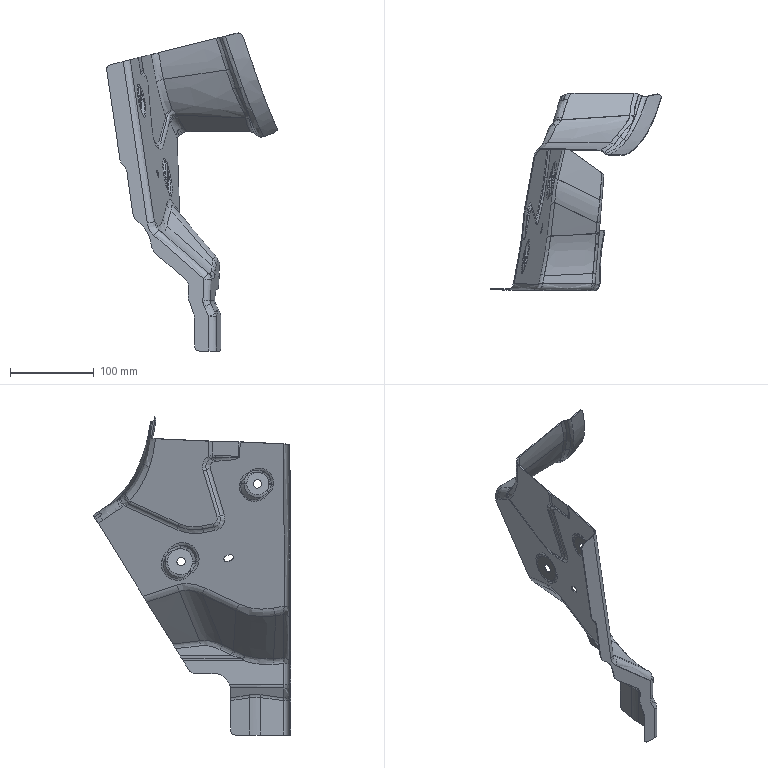Part | STEP file | FNA5401755 | 1 solid | 330 faces | box 204.272 x 236.4 x 380.596 mm | volume 84928 mm3 | spline 251 | cylinder 46 | plane 28 | other 3 | sphere 2 | commonest cylinder face diameters 17.6 x7 15.6 x6 10 x4 18.4 x4 20.4 x4 10.4 x3